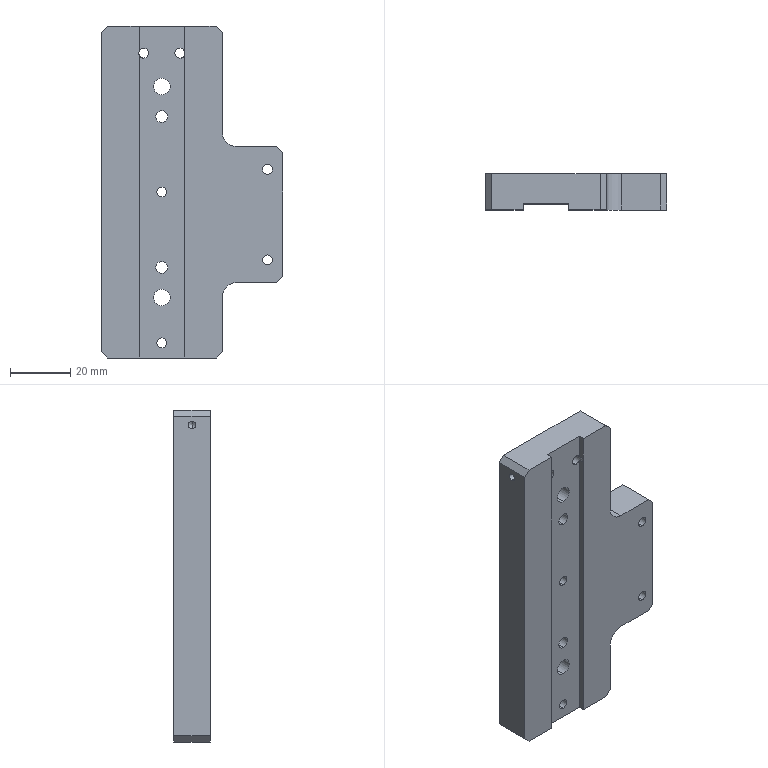Part | STEP file | PN_0001 | 1 solid | 73 faces | box 60 x 12 x 110 mm | volume 56528 mm3 | cylinder 37 | plane 28 | cone 8 | commonest cylinder face diameters 3.3 x12 3 x7 10 x6 2.5 x4 4 x4 5.5 x4